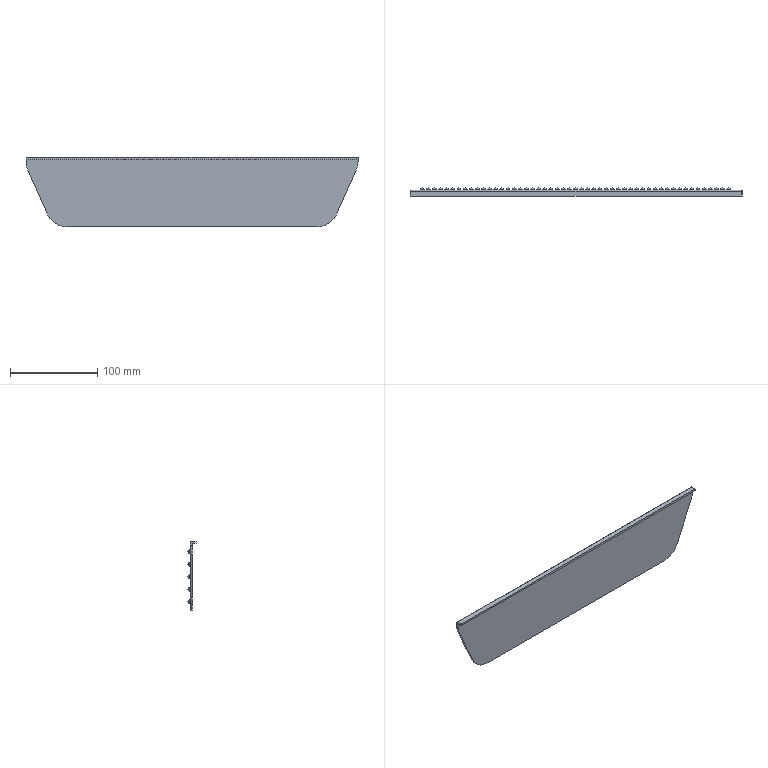Part | STEP file | Plastic anti-slip plate | 1 solid | 257 faces | box 380 x 9.3 x 80 mm | volume 74474 mm3 | cylinder 127 | sphere 120 | plane 10 | commonest cylinder face diameters 4.5 x120 50 x4 2 x2 4.263 x1